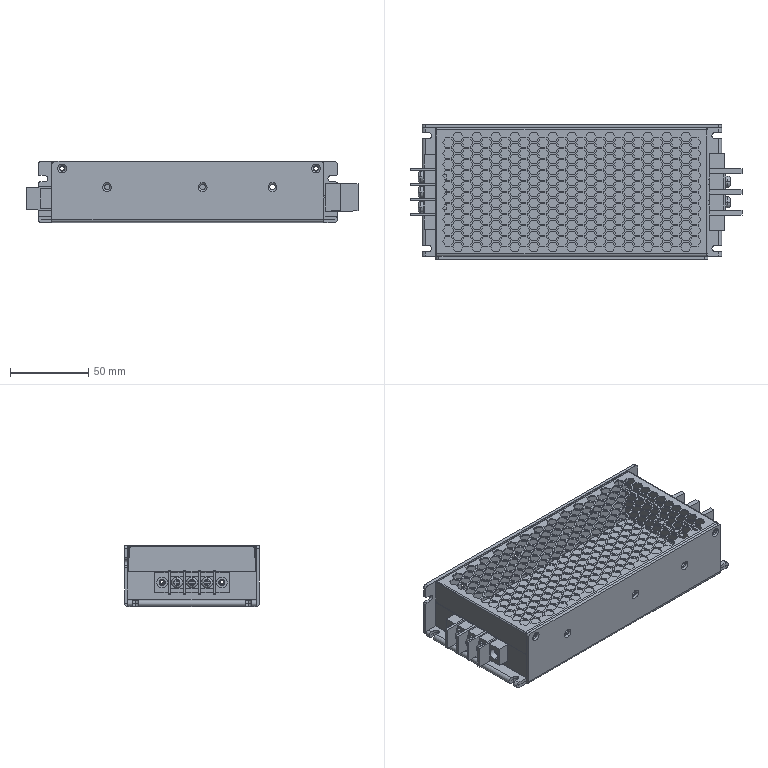Part | 3 solids | 2200 faces | box 211.801 x 86 x 39 mm | volume 87691 mm3 | plane 2021 | cylinder 133 | torus 26 | cone 20 | commonest cylinder face diameters 3.4 x20 4.2 x19 4 x16 7 x10 2 x8 2.6 x8